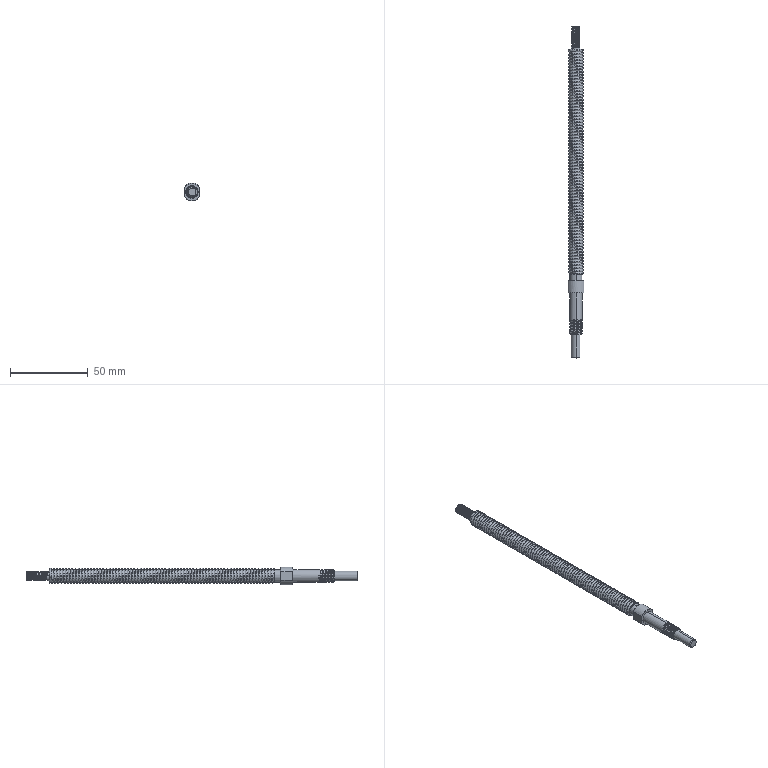Part | NX | features BREP 1 | 1 solid | 271 faces | box 10 x 214 x 11.5 mm | volume 11752 mm3 | cylinder 218 | plane 28 | cone 20 | spline 5 | commonest cylinder face diameters 10 x146 6 x45 8 x22 11.5 x3 4.917 x1 6.917 x1